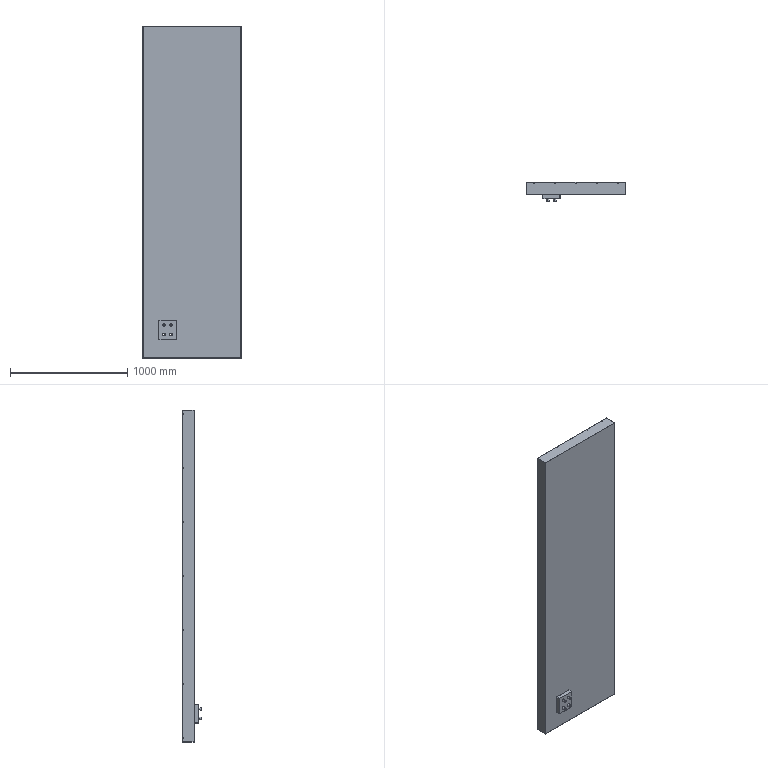Part | SolidWorks | features ICE 6, 3DProfileFeature 3, HoleWzd 3, LPattern 2, Fillet 1, FlatPattern 1, SMBaseFlange 1, SheetMetal 1 | 4 solids | 145 faces | box 840 x 159 x 2830 mm | volume 3143571 mm3 | cylinder 92 | plane 53 | commonest cylinder face diameters 4.8 x48 24 x16 4 x10 6 x10 19 x8